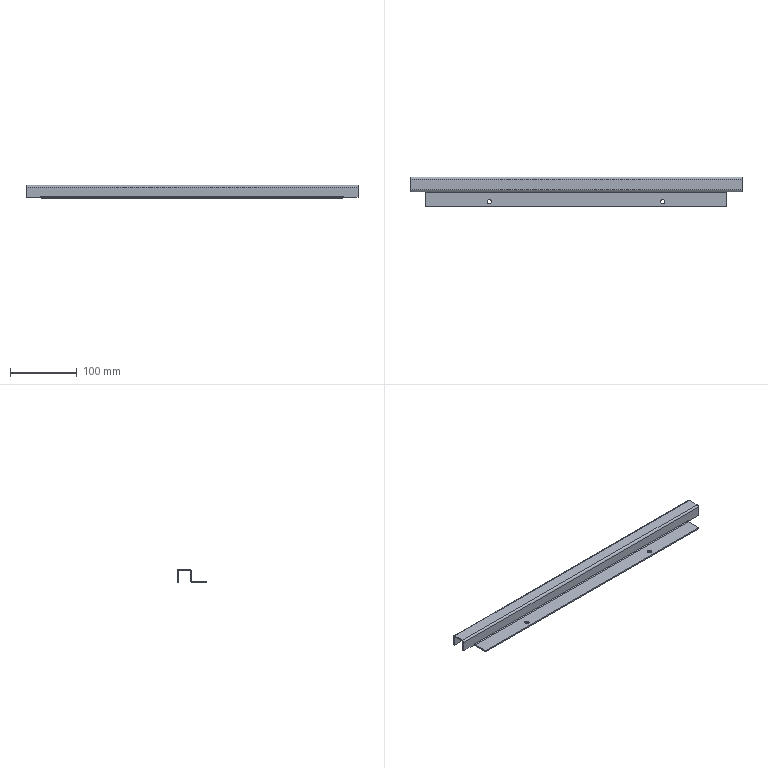Part | SolidWorks | features BaseBody 1 | 1 solid | 44 faces | box 498 x 44.9 x 20 mm | volume 75466 mm3 | plane 34 | cylinder 10 | commonest cylinder face diameters 6.5 x4 2 x3 6 x3
STEP:
#1=CARTESIAN_POINT('',(-226.,8.95,-18.));
#2=VERTEX_POINT('',#1);
#3=CARTESIAN_POINT('',(-226.,10.95,-18.));
#4=VERTEX_POINT('',#3);
#5=CARTESIAN_POINT('',(-226.,-33.95,-18.));
#6=DIRECTION('',(0.,1.,0.));
#7=VECTOR('',#6,1000.);
#8=LINE('',#5,#7);
#9=EDGE_CURVE('',#2,#4,#8,.T.);
#10=ORIENTED_EDGE('',*,*,#9,.T.);
#11=CARTESIAN_POINT('',(-226.,10.95,-20.));
#12=VERTEX_POINT('',#11);
#13=CARTESIAN_POINT('',(-226.,10.95,-20.));
#14=DIRECTION('',(0.,0.,-1.));
#15=VECTOR('',#14,1000.);
#16=LINE('',#13,#15);
#17=EDGE_CURVE('',#4,#12,#16,.T.);
#18=ORIENTED_EDGE('',*,*,#17,.T.);
#19=CARTESIAN_POINT('',(-226.,8.95,-20.));
#20=VERTEX_POINT('',#19);
#21=CARTESIAN_POINT('',(-226.,-33.95,-20.));
#22=DIRECTION('',(0.,1.,0.));
#23=VECTOR('',#22,1000.);
#24=LINE('',#21,#23);
#25=EDGE_CURVE('',#20,#12,#24,.T.);
#26=ORIENTED_EDGE('',*,*,#25,.F.);
#27=CARTESIAN_POINT('',(-226.,8.95,0.));
#28=DIRECTION('',(0.,0.,-1.));
#29=VECTOR('',#28,1000.);
#30=LINE('',#27,#29);
#31=EDGE_CURVE('',#2,#20,#30,.T.);
#32=ORIENTED_EDGE('',*,*,#31,.F.);
#33=EDGE_LOOP('',(#10,#18,#26,#32));
#34=FACE_OUTER_BOUND('',#33,.T.);
#35=CARTESIAN_POINT('',(-226.,-33.95,-20.));
#36=DIRECTION('',(1.,0.,0.));
#37=DIRECTION('',(0.,1.,0.));
#38=AXIS2_PLACEMENT_3D('',#35,#36,#37);
#39=PLANE('',#38);
#40=ADVANCED_FACE('',(#34),#39,.F.);
#41=CARTESIAN_POINT('',(-249.,8.95,-18.));
#42=VERTEX_POINT('',#41);
#43=CARTESIAN_POINT('',(-249.,10.95,-18.));
#44=VERTEX_POINT('',#43);
#45=CARTESIAN_POINT('',(-249.,-33.95,-18.));
#46=DIRECTION('',(0.,1.,0.));
#47=VECTOR('',#46,1000.);
#48=LINE('',#45,#47);
#49=EDGE_CURVE('',#42,#44,#48,.T.);
#50=ORIENTED_EDGE('',*,*,#49,.T.);
#51=CARTESIAN_POINT('',(-249.,10.95,-18.));
#52=DIRECTION('',(1.,0.,0.));
#53=VECTOR('',#52,1000.);
#54=LINE('',#51,#53);
#55=EDGE_CURVE('',#44,#4,#54,.T.);
#56=ORIENTED_EDGE('',*,*,#55,.T.);
#57=ORIENTED_EDGE('',*,*,#9,.F.);
#58=CARTESIAN_POINT('',(0.,8.95,-18.));
#59=DIRECTION('',(1.,0.,0.));
#60=VECTOR('',#59,1000.);
#61=LINE('',#58,#60);
#62=EDGE_CURVE('',#42,#2,#61,.T.);
#63=ORIENTED_EDGE('',*,*,#62,.F.);
#64=EDGE_LOOP('',(#50,#56,#57,#63));
#65=FACE_OUTER_BOUND('',#64,.T.);
#66=CARTESIAN_POINT('',(-249.,-33.95,-18.));
#67=DIRECTION('',(0.,0.,1.));
#68=DIRECTION('',(0.,-1.,0.));
#69=AXIS2_PLACEMENT_3D('',#66,#67,#68);
#70=PLANE('',#69);
#71=ADVANCED_FACE('',(#65),#70,.F.);
#72=CARTESIAN_POINT('',(226.,8.95,-20.));
#73=VERTEX_POINT('',#72);
#74=CARTESIAN_POINT('',(226.,10.95,-20.));
#75=VERTEX_POINT('',#74);
#76=CARTESIAN_POINT('',(226.,-33.95,-20.));
#77=DIRECTION('',(0.,1.,0.));
#78=VECTOR('',#77,1000.);
#79=LINE('',#76,#78);
#80=EDGE_CURVE('',#73,#75,#79,.T.);
#81=ORIENTED_EDGE('',*,*,#80,.T.);
#82=CARTESIAN_POINT('',(226.,10.95,-18.));
#83=VERTEX_POINT('',#82);
#84=CARTESIAN_POINT('',(226.,10.95,-20.));
#85=DIRECTION('',(0.,0.,1.));
#86=VECTOR('',#85,1000.);
#87=LINE('',#84,#86);
#88=EDGE_CURVE('',#75,#83,#87,.T.);
#89=ORIENTED_EDGE('',*,*,#88,.T.);
#90=CARTESIAN_POINT('',(226.,8.95,-18.));
#91=VERTEX_POINT('',#90);
#92=CARTESIAN_POINT('',(226.,-33.95,-18.));
#93=DIRECTION('',(0.,1.,0.));
#94=VECTOR('',#93,1000.);
#95=LINE('',#92,#94);
#96=EDGE_CURVE('',#91,#83,#95,.T.);
#97=ORIENTED_EDGE('',*,*,#96,.F.);
#98=CARTESIAN_POINT('',(226.,8.95,0.));
#99=DIRECTION('',(0.,0.,1.));
#100=VECTOR('',#99,1000.);
#101=LINE('',#98,#100);
#102=EDGE_CURVE('',#73,#91,#101,.T.);
#103=ORIENTED_EDGE('',*,*,#102,.F.);
#104=EDGE_LOOP('',(#81,#89,#97,#103));
#105=FACE_OUTER_BOUND('',#104,.T.);
#106=CARTESIAN_POINT('',(226.,-33.95,-20.));
#107=DIRECTION('',(-1.,0.,0.));
#108=DIRECTION('',(0.,0.,1.));
#109=AXIS2_PLACEMENT_3D('',#106,#107,#108);
#110=PLANE('',#109);
#111=ADVANCED_FACE('',(#105),#110,.F.);
#112=ORIENTED_EDGE('',*,*,#96,.T.);
#113=CARTESIAN_POINT('',(249.,10.95,-18.));
#114=VERTEX_POINT('',#113);
#115=CARTESIAN_POINT('',(249.,10.95,-18.));
#116=DIRECTION('',(1.,0.,0.));
#117=VECTOR('',#116,1000.);
#118=LINE('',#115,#117);
#119=EDGE_CURVE('',#83,#114,#118,.T.);
#120=ORIENTED_EDGE('',*,*,#119,.T.);
#121=CARTESIAN_POINT('',(249.,8.95,-18.));
#122=VERTEX_POINT('',#121);
#123=CARTESIAN_POINT('',(249.,-33.95,-18.));
#124=DIRECTION('',(0.,1.,0.));
#125=VECTOR('',#124,1000.);
#126=LINE('',#123,#125);
#127=EDGE_CURVE('',#122,#114,#126,.T.);
#128=ORIENTED_EDGE('',*,*,#127,.F.);
#129=CARTESIAN_POINT('',(0.,8.95,-18.));
#130=DIRECTION('',(1.,0.,0.));
#131=VECTOR('',#130,1000.);
#132=LINE('',#129,#131);
#133=EDGE_CURVE('',#91,#122,#132,.T.);
#134=ORIENTED_EDGE('',*,*,#133,.F.);
#135=EDGE_LOOP('',(#112,#120,#128,#134));
#136=FACE_OUTER_BOUND('',#135,.T.);
#137=CARTESIAN_POINT('',(249.,-33.95,-18.));
#138=DIRECTION('',(0.,0.,1.));
#139=DIRECTION('',(0.,-1.,0.));
#140=AXIS2_PLACEMENT_3D('',#137,#138,#139);
#141=PLANE('',#140);
#142=ADVANCED_FACE('',(#136),#141,.F.);
#143=CARTESIAN_POINT('',(227.,-10.95,-18.));
#144=VERTEX_POINT('',#143);
#145=CARTESIAN_POINT('',(227.,-8.95,-18.));
#146=VERTEX_POINT('',#145);
#147=CARTESIAN_POINT('',(227.,-10.95,-18.));
#148=DIRECTION('',(0.,1.,0.));
#149=VECTOR('',#148,1000.);
#150=LINE('',#147,#149);
#151=EDGE_CURVE('',#144,#146,#150,.T.);
#152=ORIENTED_EDGE('',*,*,#151,.T.);
#153=CARTESIAN_POINT('',(249.,-8.95,-18.));
#154=VERTEX_POINT('',#153);
#155=CARTESIAN_POINT('',(0.,-8.95,-18.));
#156=DIRECTION('',(1.,0.,0.));
#157=VECTOR('',#156,1000.);
#158=LINE('',#155,#157);
#159=EDGE_CURVE('',#146,#154,#158,.T.);
#160=ORIENTED_EDGE('',*,*,#159,.T.);
#161=CARTESIAN_POINT('',(249.,-10.95,-18.));
#162=VERTEX_POINT('',#161);
#163=CARTESIAN_POINT('',(249.,-33.95,-18.));
#164=DIRECTION('',(0.,1.,0.));
#165=VECTOR('',#164,1000.);
#166=LINE('',#163,#165);
#167=EDGE_CURVE('',#162,#154,#166,.T.);
#168=ORIENTED_EDGE('',*,*,#167,.F.);
#169=CARTESIAN_POINT('',(0.,-10.95,-18.));
#170=DIRECTION('',(1.,0.,0.));
#171=VECTOR('',#170,1000.);
#172=LINE('',#169,#171);
#173=EDGE_CURVE('',#144,#162,#172,.T.);
#174=ORIENTED_EDGE('',*,*,#173,.F.);
#175=EDGE_LOOP('',(#152,#160,#168,#174));
#176=FACE_OUTER_BOUND('',#175,.T.);
#177=CARTESIAN_POINT('',(249.,-33.95,-18.));
#178=DIRECTION('',(0.,0.,1.));
#179=DIRECTION('',(0.,-1.,0.));
#180=AXIS2_PLACEMENT_3D('',#177,#178,#179);
#181=PLANE('',#180);
#182=ADVANCED_FACE('',(#176),#181,.F.);
#183=CARTESIAN_POINT('',(-249.,-10.95,-18.));
#184=VERTEX_POINT('',#183);
#185=CARTESIAN_POINT('',(-249.,-8.95,-18.));
#186=VERTEX_POINT('',#185);
#187=CARTESIAN_POINT('',(-249.,-33.95,-18.));
#188=DIRECTION('',(0.,1.,0.));
#189=VECTOR('',#188,1000.);
#190=LINE('',#187,#189);
#191=EDGE_CURVE('',#184,#186,#190,.T.);
#192=ORIENTED_EDGE('',*,*,#191,.T.);
#193=CARTESIAN_POINT('',(-227.,-8.95,-18.));
#194=VERTEX_POINT('',#193);
#195=CARTESIAN_POINT('',(0.,-8.95,-18.));
#196=DIRECTION('',(1.,0.,0.));
#197=VECTOR('',#196,1000.);
#198=LINE('',#195,#197);
#199=EDGE_CURVE('',#186,#194,#198,.T.);
#200=ORIENTED_EDGE('',*,*,#199,.T.);
#201=CARTESIAN_POINT('',(-227.,-10.95,-18.));
#202=VERTEX_POINT('',#201);
#203=CARTESIAN_POINT('',(-227.,-10.95,-18.));
#204=DIRECTION('',(0.,-1.,0.));
#205=VECTOR('',#204,1000.);
#206=LINE('',#203,#205);
#207=EDGE_CURVE('',#194,#202,#206,.T.);
#208=ORIENTED_EDGE('',*,*,#207,.T.);
#209=CARTESIAN_POINT('',(0.,-10.95,-18.));
#210=DIRECTION('',(1.,0.,0.));
#211=VECTOR('',#210,1000.);
#212=LINE('',#209,#211);
#213=EDGE_CURVE('',#184,#202,#212,.T.);
#214=ORIENTED_EDGE('',*,*,#213,.F.);
#215=EDGE_LOOP('',(#192,#200,#208,#214));
#216=FACE_OUTER_BOUND('',#215,.T.);
#217=CARTESIAN_POINT('',(-249.,-33.95,-18.));
#218=DIRECTION('',(0.,0.,1.));
#219=DIRECTION('',(0.,-1.,0.));
#220=AXIS2_PLACEMENT_3D('',#217,#218,#219);
#221=PLANE('',#220);
#222=ADVANCED_FACE('',(#216),#221,.F.);
#223=CARTESIAN_POINT('',(-133.25,-25.95,-20.));
#224=VERTEX_POINT('',#223);
#225=CARTESIAN_POINT('',(-133.25,-25.95,-18.));
#226=VERTEX_POINT('',#225);
#227=CARTESIAN_POINT('',(-133.25,-25.95,-20.));
#228=DIRECTION('',(0.,0.,1.));
#229=VECTOR('',#228,1000.);
#230=LINE('',#227,#229);
#231=EDGE_CURVE('',#224,#226,#230,.T.);
#232=ORIENTED_EDGE('',*,*,#231,.F.);
#233=CARTESIAN_POINT('',(-126.75,-25.95,-20.));
#234=VERTEX_POINT('',#233);
#235=CARTESIAN_POINT('',(-130.,-25.95,-20.));
#236=DIRECTION('',(0.,0.,1.));
#237=DIRECTION('',(1.,0.,0.));
#238=AXIS2_PLACEMENT_3D('',#235,#236,#237);
#239=CIRCLE('',#238,3.25);
#240=EDGE_CURVE('',#234,#224,#239,.T.);
#241=ORIENTED_EDGE('',*,*,#240,.F.);
#242=CARTESIAN_POINT('',(-126.75,-25.95,-18.));
#243=VERTEX_POINT('',#242);
#244=CARTESIAN_POINT('',(-126.75,-25.95,-20.));
#245=DIRECTION('',(0.,0.,1.));
#246=VECTOR('',#245,1000.);
#247=LINE('',#244,#246);
#248=EDGE_CURVE('',#234,#243,#247,.T.);
#249=ORIENTED_EDGE('',*,*,#248,.T.);
#250=CARTESIAN_POINT('',(-130.,-25.95,-18.));
#251=DIRECTION('',(0.,0.,1.));
#252=DIRECTION('',(1.,0.,0.));
#253=AXIS2_PLACEMENT_3D('',#250,#251,#252);
#254=CIRCLE('',#253,3.25);
#255=EDGE_CURVE('',#243,#226,#254,.T.);
#256=ORIENTED_EDGE('',*,*,#255,.T.);
#257=EDGE_LOOP('',(#232,#241,#249,#256));
#258=FACE_OUTER_BOUND('',#257,.T.);
#259=CARTESIAN_POINT('',(-130.,-25.95,-20.));
#260=DIRECTION('',(0.,0.,1.));
#261=DIRECTION('',(1.,0.,0.));
#262=AXIS2_PLACEMENT_3D('',#259,#260,#261);
#263=CYLINDRICAL_SURFACE('',#262,3.25);
#264=ADVANCED_FACE('',(#258),#263,.F.);
#265=CARTESIAN_POINT('',(126.75,-25.95,-20.));
#266=VERTEX_POINT('',#265);
#267=CARTESIAN_POINT('',(126.75,-25.95,-18.));
#268=VERTEX_POINT('',#267);
#269=CARTESIAN_POINT('',(126.75,-25.95,-20.));
#270=DIRECTION('',(0.,0.,1.));
#271=VECTOR('',#270,1000.);
#272=LINE('',#269,#271);
#273=EDGE_CURVE('',#266,#268,#272,.T.);
#274=ORIENTED_EDGE('',*,*,#273,.F.);
#275=CARTESIAN_POINT('',(133.25,-25.95,-20.));
#276=VERTEX_POINT('',#275);
#277=CARTESIAN_POINT('',(130.,-25.95,-20.));
#278=DIRECTION('',(0.,0.,1.));
#279=DIRECTION('',(-1.,0.,0.));
#280=AXIS2_PLACEMENT_3D('',#277,#278,#279);
#281=CIRCLE('',#280,3.25);
#282=EDGE_CURVE('',#276,#266,#281,.T.);
#283=ORIENTED_EDGE('',*,*,#282,.F.);
#284=CARTESIAN_POINT('',(133.25,-25.95,-18.));
#285=VERTEX_POINT('',#284);
#286=CARTESIAN_POINT('',(133.25,-25.95,-20.));
#287=DIRECTION('',(0.,0.,1.));
#288=VECTOR('',#287,1000.);
#289=LINE('',#286,#288);
#290=EDGE_CURVE('',#276,#285,#289,.T.);
#291=ORIENTED_EDGE('',*,*,#290,.T.);
#292=CARTESIAN_POINT('',(130.,-25.95,-18.));
#293=DIRECTION('',(0.,0.,1.));
#294=DIRECTION('',(-1.,0.,0.));
#295=AXIS2_PLACEMENT_3D('',#292,#293,#294);
#296=CIRCLE('',#295,3.25);
#297=EDGE_CURVE('',#285,#268,#296,.T.);
#298=ORIENTED_EDGE('',*,*,#297,.T.);
#299=EDGE_LOOP('',(#274,#283,#291,#298));
#300=FACE_OUTER_BOUND('',#299,.T.);
#301=CARTESIAN_POINT('',(130.,-25.95,-20.));
#302=DIRECTION('',(0.,0.,1.));
#303=DIRECTION('',(1.,0.,0.));
#304=AXIS2_PLACEMENT_3D('',#301,#302,#303);
#305=CYLINDRICAL_SURFACE('',#304,3.25);
#306=ADVANCED_FACE('',(#300),#305,.F.);
#307=CARTESIAN_POINT('',(-226.,-33.95,-18.));
#308=VERTEX_POINT('',#307);
#309=CARTESIAN_POINT('',(226.,-33.95,-18.));
#310=VERTEX_POINT('',#309);
#311=CARTESIAN_POINT('',(0.,-33.95,-18.));
#312=DIRECTION('',(1.,0.,0.));
#313=VECTOR('',#312,1000.);
#314=LINE('',#311,#313);
#315=EDGE_CURVE('',#308,#310,#314,.T.);
#316=ORIENTED_EDGE('',*,*,#315,.F.);
#317=CARTESIAN_POINT('',(-226.,-33.95,-20.));
#318=VERTEX_POINT('',#317);
#319=CARTESIAN_POINT('',(-226.,-33.95,-20.));
#320=DIRECTION('',(0.,0.,1.));
#321=VECTOR('',#320,1000.);
#322=LINE('',#319,#321);
#323=EDGE_CURVE('',#318,#308,#322,.T.);
#324=ORIENTED_EDGE('',*,*,#323,.F.);
#325=CARTESIAN_POINT('',(226.,-33.95,-20.));
#326=VERTEX_POINT('',#325);
#327=CARTESIAN_POINT('',(-226.,-33.95,-20.));
#328=DIRECTION('',(1.,0.,0.));
#329=VECTOR('',#328,1000.);
#330=LINE('',#327,#329);
#331=EDGE_CURVE('',#318,#326,#330,.T.);
#332=ORIENTED_EDGE('',*,*,#331,.T.);
#333=CARTESIAN_POINT('',(226.,-33.95,-20.));
#334=DIRECTION('',(0.,0.,1.));
#335=VECTOR('',#334,1000.);
#336=LINE('',#333,#335);
#337=EDGE_CURVE('',#326,#310,#336,.T.);
#338=ORIENTED_EDGE('',*,*,#337,.T.);
#339=EDGE_LOOP('',(#316,#324,#332,#338));
#340=FACE_OUTER_BOUND('',#339,.T.);
#341=CARTESIAN_POINT('',(-226.,-33.95,-20.));
#342=DIRECTION('',(0.,-1.,0.));
#343=DIRECTION('',(0.,0.,-1.));
#344=AXIS2_PLACEMENT_3D('',#341,#342,#343);
#345=PLANE('',#344);
#346=ADVANCED_FACE('',(#340),#345,.T.);
#347=ORIENTED_EDGE('',*,*,#297,.F.);
#348=CARTESIAN_POINT('',(130.,-25.95,-18.));
#349=DIRECTION('',(0.,0.,1.));
#350=DIRECTION('',(-1.,0.,0.));
#351=AXIS2_PLACEMENT_3D('',#348,#349,#350);
#352=CIRCLE('',#351,3.25);
#353=EDGE_CURVE('',#268,#285,#352,.T.);
#354=ORIENTED_EDGE('',*,*,#353,.F.);
#355=EDGE_LOOP('',(#347,#354));
#356=FACE_BOUND('',#355,.T.);
#357=ORIENTED_EDGE('',*,*,#255,.F.);
#358=CARTESIAN_POINT('',(-130.,-25.95,-18.));
#359=DIRECTION('',(0.,0.,1.));
#360=DIRECTION('',(1.,0.,0.));
#361=AXIS2_PLACEMENT_3D('',#358,#359,#360);
#362=CIRCLE('',#361,3.25);
#363=EDGE_CURVE('',#226,#243,#362,.T.);
#364=ORIENTED_EDGE('',*,*,#363,.F.);
#365=EDGE_LOOP('',(#357,#364));
#366=FACE_BOUND('',#365,.T.);
#367=CARTESIAN_POINT('',(226.,-11.95,-18.));
#368=VERTEX_POINT('',#367);
#369=CARTESIAN_POINT('',(226.,0.,-18.));
#370=DIRECTION('',(0.,1.,0.));
#371=VECTOR('',#370,1000.);
#372=LINE('',#369,#371);
#373=EDGE_CURVE('',#310,#368,#372,.T.);
#374=ORIENTED_EDGE('',*,*,#373,.T.);
#375=CARTESIAN_POINT('',(-226.,-11.95,-18.));
#376=VERTEX_POINT('',#375);
#377=CARTESIAN_POINT('',(-226.,-11.95,-18.));
#378=DIRECTION('',(1.,0.,0.));
#379=VECTOR('',#378,1000.);
#380=LINE('',#377,#379);
#381=EDGE_CURVE('',#376,#368,#380,.T.);
#382=ORIENTED_EDGE('',*,*,#381,.F.);
#383=CARTESIAN_POINT('',(-226.,0.,-18.));
#384=DIRECTION('',(0.,-1.,0.));
#385=VECTOR('',#384,1000.);
#386=LINE('',#383,#385);
#387=EDGE_CURVE('',#376,#308,#386,.T.);
#388=ORIENTED_EDGE('',*,*,#387,.T.);
#389=ORIENTED_EDGE('',*,*,#315,.T.);
#390=EDGE_LOOP('',(#374,#382,#388,#389));
#391=FACE_OUTER_BOUND('',#390,.T.);
#392=CARTESIAN_POINT('',(0.,0.,-18.));
#393=DIRECTION('',(0.,0.,1.));
#394=DIRECTION('',(1.,0.,0.));
#395=AXIS2_PLACEMENT_3D('',#392,#393,#394);
#396=PLANE('',#395);
#397=ADVANCED_FACE('',(#356,#366,#391),#396,.T.);
#398=ORIENTED_EDGE('',*,*,#282,.T.);
#399=CARTESIAN_POINT('',(130.,-25.95,-20.));
#400=DIRECTION('',(0.,0.,1.));
#401=DIRECTION('',(-1.,0.,0.));
#402=AXIS2_PLACEMENT_3D('',#399,#400,#401);
#403=CIRCLE('',#402,3.25);
#404=EDGE_CURVE('',#266,#276,#403,.T.);
#405=ORIENTED_EDGE('',*,*,#404,.T.);
#406=EDGE_LOOP('',(#398,#405));
#407=FACE_BOUND('',#406,.T.);
#408=ORIENTED_EDGE('',*,*,#240,.T.);
#409=CARTESIAN_POINT('',(-130.,-25.95,-20.));
#410=DIRECTION('',(0.,0.,1.));
#411=DIRECTION('',(1.,0.,0.));
#412=AXIS2_PLACEMENT_3D('',#409,#410,#411);
#413=CIRCLE('',#412,3.25);
#414=EDGE_CURVE('',#224,#234,#413,.T.);
#415=ORIENTED_EDGE('',*,*,#414,.T.);
#416=EDGE_LOOP('',(#408,#415));
#417=FACE_BOUND('',#416,.T.);
#418=CARTESIAN_POINT('',(226.,-11.95,-20.));
#419=VERTEX_POINT('',#418);
#420=CARTESIAN_POINT('',(-226.,-11.95,-20.));
#421=VERTEX_POINT('',#420);
#422=CARTESIAN_POINT('',(-226.,-11.95,-20.));
#423=DIRECTION('',(-1.,0.,0.));
#424=VECTOR('',#423,1000.);
#425=LINE('',#422,#424);
#426=EDGE_CURVE('',#419,#421,#425,.T.);
#427=ORIENTED_EDGE('',*,*,#426,.F.);
#428=CARTESIAN_POINT('',(226.,-10.95,-20.));
#429=DIRECTION('',(0.,1.,0.));
#430=VECTOR('',#429,1000.);
#431=LINE('',#428,#430);
#432=EDGE_CURVE('',#326,#419,#431,.T.);
#433=ORIENTED_EDGE('',*,*,#432,.F.);
#434=ORIENTED_EDGE('',*,*,#331,.F.);
#435=CARTESIAN_POINT('',(-226.,-10.95,-20.));
#436=DIRECTION('',(0.,-1.,0.));
#437=VECTOR('',#436,1000.);
#438=LINE('',#435,#437);
#439=EDGE_CURVE('',#421,#318,#438,.T.);
#440=ORIENTED_EDGE('',*,*,#439,.F.);
#441=EDGE_LOOP('',(#427,#433,#434,#440));
#442=FACE_OUTER_BOUND('',#441,.T.);
#443=CARTESIAN_POINT('',(0.,0.,-20.));
#444=DIRECTION('',(0.,0.,1.));
#445=DIRECTION('',(1.,0.,0.));
#446=AXIS2_PLACEMENT_3D('',#443,#444,#445);
#447=PLANE('',#446);
#448=ADVANCED_FACE('',(#407,#417,#442),#447,.F.);
#449=CARTESIAN_POINT('',(226.,-10.95,-17.));
#450=VERTEX_POINT('',#449);
#451=CARTESIAN_POINT('',(-226.,-10.95,-17.));
#452=VERTEX_POINT('',#451);
#453=CARTESIAN_POINT('',(226.,-10.95,-17.));
#454=DIRECTION('',(-1.,0.,0.));
#455=VECTOR('',#454,1000.);
#456=LINE('',#453,#455);
#457=EDGE_CURVE('',#450,#452,#456,.T.);
#458=ORIENTED_EDGE('',*,*,#457,.T.);
#459=CARTESIAN_POINT('',(-226.,-11.95,-17.));
#460=DIRECTION('',(-1.,0.,0.));
#461=DIRECTION('',(0.,0.,-1.));
#462=AXIS2_PLACEMENT_3D('',#459,#460,#461);
#463=CIRCLE('',#462,1.);
#464=EDGE_CURVE('',#452,#376,#463,.T.);
#465=ORIENTED_EDGE('',*,*,#464,.T.);
#466=ORIENTED_EDGE('',*,*,#381,.T.);
#467=CARTESIAN_POINT('',(226.,-11.95,-17.));
#468=DIRECTION('',(1.,0.,0.));
#469=DIRECTION('',(0.,0.,-1.));
#470=AXIS2_PLACEMENT_3D('',#467,#468,#469);
#471=CIRCLE('',#470,1.);
#472=EDGE_CURVE('',#368,#450,#471,.T.);
#473=ORIENTED_EDGE('',*,*,#472,.T.);
#474=EDGE_LOOP('',(#458,#465,#466,#473));
#475=FACE_OUTER_BOUND('',#474,.T.);
#476=CARTESIAN_POINT('',(226.,-11.95,-17.));
#477=DIRECTION('',(1.,0.,0.));
#478=DIRECTION('',(0.,0.,-1.));
#479=AXIS2_PLACEMENT_3D('',#476,#477,#478);
#480=CYLINDRICAL_SURFACE('',#479,1.);
#481=ADVANCED_FACE('',(#475),#480,.F.);
#482=CARTESIAN_POINT('',(226.,-8.95,-17.));
#483=VERTEX_POINT('',#482);
#484=CARTESIAN_POINT('',(-226.,-8.95,-17.));
#485=VERTEX_POINT('',#484);
#486=CARTESIAN_POINT('',(226.,-8.95,-17.));
#487=DIRECTION('',(-1.,0.,0.));
#488=VECTOR('',#487,1000.);
#489=LINE('',#486,#488);
#490=EDGE_CURVE('',#483,#485,#489,.T.);
#491=ORIENTED_EDGE('',*,*,#490,.F.);
#492=CARTESIAN_POINT('',(226.,-11.95,-17.));
#493=DIRECTION('',(1.,0.,0.));
#494=DIRECTION('',(0.,0.,-1.));
#495=AXIS2_PLACEMENT_3D('',#492,#493,#494);
#496=CIRCLE('',#495,3.);
#497=EDGE_CURVE('',#419,#483,#496,.T.);
#498=ORIENTED_EDGE('',*,*,#497,.F.);
#499=ORIENTED_EDGE('',*,*,#426,.T.);
#500=CARTESIAN_POINT('',(-226.,-11.95,-17.));
#501=DIRECTION('',(-1.,0.,0.));
#502=DIRECTION('',(0.,0.,-1.));
#503=AXIS2_PLACEMENT_3D('',#500,#501,#502);
#504=CIRCLE('',#503,3.);
#505=EDGE_CURVE('',#485,#421,#504,.T.);
#506=ORIENTED_EDGE('',*,*,#505,.F.);
#507=EDGE_LOOP('',(#491,#498,#499,#506));
#508=FACE_OUTER_BOUND('',#507,.T.);
#509=CARTESIAN_POINT('',(226.,-11.95,-17.));
#510=DIRECTION('',(1.,0.,0.));
#511=DIRECTION('',(0.,0.,-1.));
#512=AXIS2_PLACEMENT_3D('',#509,#510,#511);
#513=CYLINDRICAL_SURFACE('',#512,3.);
#514=ADVANCED_FACE('',(#508),#513,.T.);
#515=ORIENTED_EDGE('',*,*,#472,.F.);
#516=ORIENTED_EDGE('',*,*,#373,.F.);
#517=ORIENTED_EDGE('',*,*,#337,.F.);
#518=ORIENTED_EDGE('',*,*,#432,.T.);
#519=ORIENTED_EDGE('',*,*,#497,.T.);
#520=CARTESIAN_POINT('',(226.,-10.95,-17.));
#521=DIRECTION('',(0.,1.,0.));
#522=VECTOR('',#521,1000.);
#523=LINE('',#520,#522);
#524=EDGE_CURVE('',#450,#483,#523,.T.);
#525=ORIENTED_EDGE('',*,*,#524,.F.);
#526=EDGE_LOOP('',(#515,#516,#517,#518,#519,#525));
#527=FACE_OUTER_BOUND('',#526,.T.);
#528=CARTESIAN_POINT('',(226.,-11.95,-17.));
#529=DIRECTION('',(-1.,0.,0.));
#530=DIRECTION('',(0.,0.,1.));
#531=AXIS2_PLACEMENT_3D('',#528,#529,#530);
#532=PLANE('',#531);
#533=ADVANCED_FACE('',(#527),#532,.F.);
#534=ORIENTED_EDGE('',*,*,#505,.T.);
#535=ORIENTED_EDGE('',*,*,#439,.T.);
#536=ORIENTED_EDGE('',*,*,#323,.T.);
#537=ORIENTED_EDGE('',*,*,#387,.F.);
#538=ORIENTED_EDGE('',*,*,#464,.F.);
#539=CARTESIAN_POINT('',(-226.,-10.95,-17.));
#540=DIRECTION('',(0.,1.,0.));
#541=VECTOR('',#540,1000.);
#542=LINE('',#539,#541);
#543=EDGE_CURVE('',#452,#485,#542,.T.);
#544=ORIENTED_EDGE('',*,*,#543,.T.);
#545=EDGE_LOOP('',(#534,#535,#536,#537,#538,#544));
#546=FACE_OUTER_BOUND('',#545,.T.);
#547=CARTESIAN_POINT('',(-226.,-11.95,-17.));
#548=DIRECTION('',(-1.,0.,0.));
#549=DIRECTION('',(0.,0.,1.));
#550=AXIS2_PLACEMENT_3D('',#547,#548,#549);
#551=PLANE('',#550);
#552=ADVANCED_FACE('',(#546),#551,.T.);
#553=ORIENTED_EDGE('',*,*,#207,.F.);
#554=CARTESIAN_POINT('',(-227.,-8.95,-16.));
#555=VERTEX_POINT('',#554);
#556=CARTESIAN_POINT('',(-227.,-8.95,0.));
#557=DIRECTION('',(0.,0.,-1.));
#558=VECTOR('',#557,1000.);
#559=LINE('',#556,#558);
#560=EDGE_CURVE('',#555,#194,#559,.T.);
#561=ORIENTED_EDGE('',*,*,#560,.F.);
#562=CARTESIAN_POINT('',(-227.,-10.95,-16.));
#563=VERTEX_POINT('',#562);
#564=CARTESIAN_POINT('',(-227.,-10.95,-16.));
#565=DIRECTION('',(0.,1.,0.));
#566=VECTOR('',#565,1000.);
#567=LINE('',#564,#566);
#568=EDGE_CURVE('',#563,#555,#567,.T.);
#569=ORIENTED_EDGE('',*,*,#568,.F.);
#570=CARTESIAN_POINT('',(-227.,-10.95,-16.));
#571=DIRECTION('',(0.,0.,-1.));
#572=VECTOR('',#571,1000.);
#573=LINE('',#570,#572);
#574=EDGE_CURVE('',#563,#202,#573,.T.);
#575=ORIENTED_EDGE('',*,*,#574,.T.);
#576=EDGE_LOOP('',(#553,#561,#569,#575));
#577=FACE_OUTER_BOUND('',#576,.T.);
#578=CARTESIAN_POINT('',(-227.,-10.95,-16.));
#579=DIRECTION('',(1.,0.,0.));
#580=DIRECTION('',(0.,0.,1.));
#581=AXIS2_PLACEMENT_3D('',#578,#579,#580);
#582=PLANE('',#581);
#583=ADVANCED_FACE('',(#577),#582,.T.);
#584=CARTESIAN_POINT('',(-226.,-8.95,-16.));
#585=VERTEX_POINT('',#584);
#586=CARTESIAN_POINT('',(0.,-8.95,-16.));
#587=DIRECTION('',(-1.,0.,0.));
#588=VECTOR('',#587,1000.);
#589=LINE('',#586,#588);
#590=EDGE_CURVE('',#585,#555,#589,.T.);
#591=ORIENTED_EDGE('',*,*,#590,.F.);
#592=CARTESIAN_POINT('',(-226.,-10.95,-16.));
#593=VERTEX_POINT('',#592);
#594=CARTESIAN_POINT('',(-226.,-10.95,-16.));
#595=DIRECTION('',(0.,1.,0.));
#596=VECTOR('',#595,1000.);
#597=LINE('',#594,#596);
#598=EDGE_CURVE('',#593,#585,#597,.T.);
#599=ORIENTED_EDGE('',*,*,#598,.F.);
#600=CARTESIAN_POINT('',(-226.,-10.95,-16.));
#601=DIRECTION('',(-1.,0.,0.));
#602=VECTOR('',#601,1000.);
#603=LINE('',#600,#602);
#604=EDGE_CURVE('',#593,#563,#603,.T.);
#605=ORIENTED_EDGE('',*,*,#604,.T.);
#606=ORIENTED_EDGE('',*,*,#568,.T.);
#607=EDGE_LOOP('',(#591,#599,#605,#606));
#608=FACE_OUTER_BOUND('',#607,.T.);
#609=CARTESIAN_POINT('',(-226.,-10.95,-16.));
#610=DIRECTION('',(0.,0.,-1.));
#611=DIRECTION('',(0.,-1.,0.));
#612=AXIS2_PLACEMENT_3D('',#609,#610,#611);
#613=PLANE('',#612);
#614=ADVANCED_FACE('',(#608),#613,.T.);
#615=CARTESIAN_POINT('',(-226.,-8.95,0.));
#616=DIRECTION('',(0.,0.,1.));
#617=VECTOR('',#616,1000.);
#618=LINE('',#615,#617);
#619=EDGE_CURVE('',#485,#585,#618,.T.);
#620=ORIENTED_EDGE('',*,*,#619,.F.);
#621=ORIENTED_EDGE('',*,*,#543,.F.);
#622=CARTESIAN_POINT('',(-226.,-10.95,-17.));
#623=DIRECTION('',(0.,0.,1.));
#624=VECTOR('',#623,1000.);
#625=LINE('',#622,#624);
#626=EDGE_CURVE('',#452,#593,#625,.T.);
#627=ORIENTED_EDGE('',*,*,#626,.T.);
#628=ORIENTED_EDGE('',*,*,#598,.T.);
#629=EDGE_LOOP('',(#620,#621,#627,#628));
#630=FACE_OUTER_BOUND('',#629,.T.);
#631=CARTESIAN_POINT('',(-226.,-10.95,-17.));
#632=DIRECTION('',(-1.,0.,0.));
#633=DIRECTION('',(0.,1.,0.));
#634=AXIS2_PLACEMENT_3D('',#631,#632,#633);
#635=PLANE('',#634);
#636=ADVANCED_FACE('',(#630),#635,.T.);
#637=CARTESIAN_POINT('',(226.,-8.95,-16.));
#638=VERTEX_POINT('',#637);
#639=CARTESIAN_POINT('',(226.,-8.95,0.));
#640=DIRECTION('',(0.,0.,-1.));
#641=VECTOR('',#640,1000.);
#642=LINE('',#639,#641);
#643=EDGE_CURVE('',#638,#483,#642,.T.);
#644=ORIENTED_EDGE('',*,*,#643,.F.);
#645=CARTESIAN_POINT('',(226.,-10.95,-16.));
#646=VERTEX_POINT('',#645);
#647=CARTESIAN_POINT('',(226.,-10.95,-16.));
#648=DIRECTION('',(0.,1.,0.));
#649=VECTOR('',#648,1000.);
#650=LINE('',#647,#649);
#651=EDGE_CURVE('',#646,#638,#650,.T.);
#652=ORIENTED_EDGE('',*,*,#651,.F.);
#653=CARTESIAN_POINT('',(226.,-10.95,-16.));
#654=DIRECTION('',(0.,0.,-1.));
#655=VECTOR('',#654,1000.);
#656=LINE('',#653,#655);
#657=EDGE_CURVE('',#646,#450,#656,.T.);
#658=ORIENTED_EDGE('',*,*,#657,.T.);
#659=ORIENTED_EDGE('',*,*,#524,.T.);
#660=EDGE_LOOP('',(#644,#652,#658,#659));
#661=FACE_OUTER_BOUND('',#660,.T.);
#662=CARTESIAN_POINT('',(226.,-10.95,-16.));
#663=DIRECTION('',(1.,0.,0.));
#664=DIRECTION('',(0.,1.,0.));
#665=AXIS2_PLACEMENT_3D('',#662,#663,#664);
#666=PLANE('',#665);
#667=ADVANCED_FACE('',(#661),#666,.T.);
#668=CARTESIAN_POINT('',(227.,-8.95,-16.));
#669=VERTEX_POINT('',#668);
#670=CARTESIAN_POINT('',(0.,-8.95,-16.));
#671=DIRECTION('',(-1.,0.,0.));
#672=VECTOR('',#671,1000.);
#673=LINE('',#670,#672);
#674=EDGE_CURVE('',#669,#638,#673,.T.);
#675=ORIENTED_EDGE('',*,*,#674,.F.);
#676=CARTESIAN_POINT('',(227.,-10.95,-16.));
#677=VERTEX_POINT('',#676);
#678=CARTESIAN_POINT('',(227.,-10.95,-16.));
#679=DIRECTION('',(0.,1.,0.));
#680=VECTOR('',#679,1000.);
#681=LINE('',#678,#680);
#682=EDGE_CURVE('',#677,#669,#681,.T.);
#683=ORIENTED_EDGE('',*,*,#682,.F.);
#684=CARTESIAN_POINT('',(227.,-10.95,-16.));
#685=DIRECTION('',(-1.,0.,0.));
#686=VECTOR('',#685,1000.);
#687=LINE('',#684,#686);
#688=EDGE_CURVE('',#677,#646,#687,.T.);
#689=ORIENTED_EDGE('',*,*,#688,.T.);
#690=ORIENTED_EDGE('',*,*,#651,.T.);
#691=EDGE_LOOP('',(#675,#683,#689,#690));
#692=FACE_OUTER_BOUND('',#691,.T.);
#693=CARTESIAN_POINT('',(227.,-10.95,-16.));
#694=DIRECTION('',(0.,0.,-1.));
#695=DIRECTION('',(0.,-1.,0.));
#696=AXIS2_PLACEMENT_3D('',#693,#694,#695);
#697=PLANE('',#696);
#698=ADVANCED_FACE('',(#692),#697,.T.);
#699=ORIENTED_EDGE('',*,*,#151,.F.);
#700=CARTESIAN_POINT('',(227.,-10.95,-20.));
#701=DIRECTION('',(0.,0.,1.));
#702=VECTOR('',#701,1000.);
#703=LINE('',#700,#702);
#704=EDGE_CURVE('',#144,#677,#703,.T.);
#705=ORIENTED_EDGE('',*,*,#704,.T.);
#706=ORIENTED_EDGE('',*,*,#682,.T.);
#707=CARTESIAN_POINT('',(227.,-8.95,0.));
#708=DIRECTION('',(0.,0.,1.));
#709=VECTOR('',#708,1000.);
#710=LINE('',#707,#709);
#711=EDGE_CURVE('',#146,#669,#710,.T.);
#712=ORIENTED_EDGE('',*,*,#711,.F.);
#713=EDGE_LOOP('',(#699,#705,#706,#712));
#714=FACE_OUTER_BOUND('',#713,.T.);
#715=CARTESIAN_POINT('',(227.,-10.95,-20.));
#716=DIRECTION('',(-1.,0.,0.));
#717=DIRECTION('',(0.,1.,0.));
#718=AXIS2_PLACEMENT_3D('',#715,#716,#717);
#719=PLANE('',#718);
#720=ADVANCED_FACE('',(#714),#719,.T.);
#721=ORIENTED_EDGE('',*,*,#191,.F.);
#722=CARTESIAN_POINT('',(-249.,-10.95,-3.));
#723=VERTEX_POINT('',#722);
#724=CARTESIAN_POINT('',(-249.,-10.95,-20.));
#725=DIRECTION('',(0.,0.,1.));
#726=VECTOR('',#725,1000.);
#727=LINE('',#724,#726);
#728=EDGE_CURVE('',#184,#723,#727,.T.);
#729=ORIENTED_EDGE('',*,*,#728,.T.);
#730=CARTESIAN_POINT('',(-249.,-8.95,-3.));
#731=VERTEX_POINT('',#730);
#732=CARTESIAN_POINT('',(-249.,-8.95,-3.));
#733=DIRECTION('',(0.,-1.,0.));
#734=VECTOR('',#733,1000.);
#735=LINE('',#732,#734);
#736=EDGE_CURVE('',#731,#723,#735,.T.);
#737=ORIENTED_EDGE('',*,*,#736,.F.);
#738=CARTESIAN_POINT('',(-249.,-8.95,0.));
#739=DIRECTION('',(0.,0.,1.));
#740=VECTOR('',#739,1000.);
#741=LINE('',#738,#740);
#742=EDGE_CURVE('',#186,#731,#741,.T.);
#743=ORIENTED_EDGE('',*,*,#742,.F.);
#744=EDGE_LOOP('',(#721,#729,#737,#743));
#745=FACE_OUTER_BOUND('',#744,.T.);
#746=CARTESIAN_POINT('',(-249.,-10.95,-20.));
#747=DIRECTION('',(-1.,0.,0.));
#748=DIRECTION('',(0.,1.,0.));
#749=AXIS2_PLACEMENT_3D('',#746,#747,#748);
#750=PLANE('',#749);
#751=ADVANCED_FACE('',(#745),#750,.T.);
#752=ORIENTED_EDGE('',*,*,#167,.T.);
#753=CARTESIAN_POINT('',(249.,-8.95,-3.));
#754=VERTEX_POINT('',#753);
#755=CARTESIAN_POINT('',(249.,-8.95,0.));
#756=DIRECTION('',(0.,0.,-1.));
#757=VECTOR('',#756,1000.);
#758=LINE('',#755,#757);
#759=EDGE_CURVE('',#754,#154,#758,.T.);
#760=ORIENTED_EDGE('',*,*,#759,.F.);
#761=CARTESIAN_POINT('',(249.,-10.95,-3.));
#762=VERTEX_POINT('',#761);
#763=CARTESIAN_POINT('',(249.,-10.95,-3.));
#764=DIRECTION('',(0.,-1.,0.));
#765=VECTOR('',#764,1000.);
#766=LINE('',#763,#765);
#767=EDGE_CURVE('',#754,#762,#766,.T.);
#768=ORIENTED_EDGE('',*,*,#767,.T.);
#769=CARTESIAN_POINT('',(249.,-10.95,-2.));
#770=DIRECTION('',(0.,0.,-1.));
#771=VECTOR('',#770,1000.);
#772=LINE('',#769,#771);
#773=EDGE_CURVE('',#762,#162,#772,.T.);
#774=ORIENTED_EDGE('',*,*,#773,.T.);
#775=EDGE_LOOP('',(#752,#760,#768,#774));
#776=FACE_OUTER_BOUND('',#775,.T.);
#777=CARTESIAN_POINT('',(249.,-10.95,-2.));
#778=DIRECTION('',(1.,0.,0.));
#779=DIRECTION('',(0.,0.,-1.));
#780=AXIS2_PLACEMENT_3D('',#777,#778,#779);
#781=PLANE('',#780);
#782=ADVANCED_FACE('',(#776),#781,.T.);
#783=CARTESIAN_POINT('',(-249.,-7.95,-2.));
#784=VERTEX_POINT('',#783);
#785=CARTESIAN_POINT('',(249.,-7.95,-2.));
#786=VERTEX_POINT('',#785);
#787=CARTESIAN_POINT('',(-249.,-7.95,-2.));
#788=DIRECTION('',(1.,0.,0.));
#789=VECTOR('',#788,1000.);
#790=LINE('',#787,#789);
#791=EDGE_CURVE('',#784,#786,#790,.T.);
#792=ORIENTED_EDGE('',*,*,#791,.T.);
#793=CARTESIAN_POINT('',(249.,-7.95,-3.));
#794=DIRECTION('',(1.,0.,0.));
#795=DIRECTION('',(0.,0.,1.));
#796=AXIS2_PLACEMENT_3D('',#793,#794,#795);
#797=CIRCLE('',#796,1.);
#798=EDGE_CURVE('',#786,#754,#797,.T.);
#799=ORIENTED_EDGE('',*,*,#798,.T.);
#800=CARTESIAN_POINT('',(249.,-8.95,-3.));
#801=DIRECTION('',(-1.,0.,0.));
#802=VECTOR('',#801,1000.);
#803=LINE('',#800,#802);
#804=EDGE_CURVE('',#754,#731,#803,.T.);
#805=ORIENTED_EDGE('',*,*,#804,.T.);
#806=CARTESIAN_POINT('',(-249.,-7.95,-3.));
#807=DIRECTION('',(-1.,0.,0.));
#808=DIRECTION('',(0.,0.,1.));
#809=AXIS2_PLACEMENT_3D('',#806,#807,#808);
#810=CIRCLE('',#809,1.);
#811=EDGE_CURVE('',#731,#784,#810,.T.);
#812=ORIENTED_EDGE('',*,*,#811,.T.);
#813=EDGE_LOOP('',(#792,#799,#805,#812));
#814=FACE_OUTER_BOUND('',#813,.T.);
#815=CARTESIAN_POINT('',(-249.,-7.95,-3.));
#816=DIRECTION('',(-1.,0.,0.));
#817=DIRECTION('',(0.,-1.,0.));
#818=AXIS2_PLACEMENT_3D('',#815,#816,#817);
#819=CYLINDRICAL_SURFACE('',#818,1.);
#820=ADVANCED_FACE('',(#814),#819,.F.);
#821=CARTESIAN_POINT('',(-249.,-7.95,0.));
#822=VERTEX_POINT('',#821);
#823=CARTESIAN_POINT('',(249.,-7.95,0.));
#824=VERTEX_POINT('',#823);
#825=CARTESIAN_POINT('',(-249.,-7.95,0.));
#826=DIRECTION('',(1.,0.,0.));
#827=VECTOR('',#826,1000.);
#828=LINE('',#825,#827);
#829=EDGE_CURVE('',#822,#824,#828,.T.);
#830=ORIENTED_EDGE('',*,*,#829,.F.);
#831=CARTESIAN_POINT('',(-249.,-7.95,-3.));
#832=DIRECTION('',(-1.,0.,0.));
#833=DIRECTION('',(0.,0.,1.));
#834=AXIS2_PLACEMENT_3D('',#831,#832,#833);
#835=CIRCLE('',#834,3.);
#836=EDGE_CURVE('',#723,#822,#835,.T.);
#837=ORIENTED_EDGE('',*,*,#836,.F.);
#838=CARTESIAN_POINT('',(249.,-10.95,-3.));
#839=DIRECTION('',(1.,0.,0.));
#840=VECTOR('',#839,1000.);
#841=LINE('',#838,#840);
#842=EDGE_CURVE('',#723,#762,#841,.T.);
#843=ORIENTED_EDGE('',*,*,#842,.T.);
#844=CARTESIAN_POINT('',(249.,-7.95,-3.));
#845=DIRECTION('',(1.,0.,0.));
#846=DIRECTION('',(0.,0.,1.));
#847=AXIS2_PLACEMENT_3D('',#844,#845,#846);
#848=CIRCLE('',#847,3.);
#849=EDGE_CURVE('',#824,#762,#848,.T.);
#850=ORIENTED_EDGE('',*,*,#849,.F.);
#851=EDGE_LOOP('',(#830,#837,#843,#850));
#852=FACE_OUTER_BOUND('',#851,.T.);
#853=CARTESIAN_POINT('',(-249.,-7.95,-3.));
#854=DIRECTION('',(-1.,0.,0.));
#855=DIRECTION('',(0.,-1.,0.));
#856=AXIS2_PLACEMENT_3D('',#853,#854,#855);
#857=CYLINDRICAL_SURFACE('',#856,3.);
#858=ADVANCED_FACE('',(#852),#857,.T.);
#859=ORIENTED_EDGE('',*,*,#811,.F.);
#860=ORIENTED_EDGE('',*,*,#736,.T.);
#861=ORIENTED_EDGE('',*,*,#836,.T.);
#862=CARTESIAN_POINT('',(-249.,-7.95,-2.));
#863=DIRECTION('',(0.,0.,1.));
#864=VECTOR('',#863,1000.);
#865=LINE('',#862,#864);
#866=EDGE_CURVE('',#784,#822,#865,.T.);
#867=ORIENTED_EDGE('',*,*,#866,.F.);
#868=EDGE_LOOP('',(#859,#860,#861,#867));
#869=FACE_OUTER_BOUND('',#868,.T.);
#870=CARTESIAN_POINT('',(-249.,-7.95,-3.));
#871=DIRECTION('',(1.,0.,0.));
#872=DIRECTION('',(0.,1.,0.));
#873=AXIS2_PLACEMENT_3D('',#870,#871,#872);
#874=PLANE('',#873);
#875=ADVANCED_FACE('',(#869),#874,.F.);
#876=ORIENTED_EDGE('',*,*,#767,.F.);
#877=ORIENTED_EDGE('',*,*,#798,.F.);
#878=CARTESIAN_POINT('',(249.,-7.95,-2.));
#879=DIRECTION('',(0.,0.,1.));
#880=VECTOR('',#879,1000.);
#881=LINE('',#878,#880);
#882=EDGE_CURVE('',#786,#824,#881,.T.);
#883=ORIENTED_EDGE('',*,*,#882,.T.);
#884=ORIENTED_EDGE('',*,*,#849,.T.);
#885=EDGE_LOOP('',(#876,#877,#883,#884));
#886=FACE_OUTER_BOUND('',#885,.T.);
#887=CARTESIAN_POINT('',(249.,-7.95,-3.));
#888=DIRECTION('',(1.,0.,0.));
#889=DIRECTION('',(0.,1.,0.));
#890=AXIS2_PLACEMENT_3D('',#887,#888,#889);
#891=PLANE('',#890);
#892=ADVANCED_FACE('',(#886),#891,.T.);
#893=ORIENTED_EDGE('',*,*,#25,.T.);
#894=CARTESIAN_POINT('',(249.,10.95,-20.));
#895=DIRECTION('',(1.,0.,0.));
#896=VECTOR('',#895,1000.);
#897=LINE('',#894,#896);
#898=EDGE_CURVE('',#12,#75,#897,.T.);
#899=ORIENTED_EDGE('',*,*,#898,.T.);
#900=ORIENTED_EDGE('',*,*,#80,.F.);
#901=CARTESIAN_POINT('',(0.,8.95,-20.));
#902=DIRECTION('',(1.,0.,0.));
#903=VECTOR('',#902,1000.);
#904=LINE('',#901,#903);
#905=EDGE_CURVE('',#20,#73,#904,.T.);
#906=ORIENTED_EDGE('',*,*,#905,.F.);
#907=EDGE_LOOP('',(#893,#899,#900,#906));
#908=FACE_OUTER_BOUND('',#907,.T.);
#909=CARTESIAN_POINT('',(249.,10.95,-20.));
#910=DIRECTION('',(0.,0.,-1.));
#911=DIRECTION('',(-1.,0.,0.));
#912=AXIS2_PLACEMENT_3D('',#909,#910,#911);
#913=PLANE('',#912);
#914=ADVANCED_FACE('',(#908),#913,.T.);
#915=ORIENTED_EDGE('',*,*,#62,.T.);
#916=ORIENTED_EDGE('',*,*,#31,.T.);
#917=ORIENTED_EDGE('',*,*,#905,.T.);
#918=ORIENTED_EDGE('',*,*,#102,.T.);
#919=ORIENTED_EDGE('',*,*,#133,.T.);
#920=CARTESIAN_POINT('',(249.,8.95,-3.));
#921=VERTEX_POINT('',#920);
#922=CARTESIAN_POINT('',(249.,8.95,0.));
#923=DIRECTION('',(0.,0.,1.));
#924=VECTOR('',#923,1000.);
#925=LINE('',#922,#924);
#926=EDGE_CURVE('',#122,#921,#925,.T.);
#927=ORIENTED_EDGE('',*,*,#926,.T.);
#928=CARTESIAN_POINT('',(-249.,8.95,-3.));
#929=VERTEX_POINT('',#928);
#930=CARTESIAN_POINT('',(-249.,8.95,-3.));
#931=DIRECTION('',(1.,0.,0.));
#932=VECTOR('',#931,1000.);
#933=LINE('',#930,#932);
#934=EDGE_CURVE('',#929,#921,#933,.T.);
#935=ORIENTED_EDGE('',*,*,#934,.F.);
#936=CARTESIAN_POINT('',(-249.,8.95,0.));
#937=DIRECTION('',(0.,0.,-1.));
#938=VECTOR('',#937,1000.);
#939=LINE('',#936,#938);
#940=EDGE_CURVE('',#929,#42,#939,.T.);
#941=ORIENTED_EDGE('',*,*,#940,.T.);
#942=EDGE_LOOP('',(#915,#916,#917,#918,#919,#927,#935,#941));
#943=FACE_OUTER_BOUND('',#942,.T.);
#944=CARTESIAN_POINT('',(0.,8.95,0.));
#945=DIRECTION('',(0.,1.,0.));
#946=DIRECTION('',(0.,0.,-1.));
#947=AXIS2_PLACEMENT_3D('',#944,#945,#946);
#948=PLANE('',#947);
#949=ADVANCED_FACE('',(#943),#948,.F.);
#950=ORIENTED_EDGE('',*,*,#17,.F.);
#951=ORIENTED_EDGE('',*,*,#55,.F.);
#952=CARTESIAN_POINT('',(-249.,10.95,-3.));
#953=VERTEX_POINT('',#952);
#954=CARTESIAN_POINT('',(-249.,10.95,-20.));
#955=DIRECTION('',(0.,0.,-1.));
#956=VECTOR('',#955,1000.);
#957=LINE('',#954,#956);
#958=EDGE_CURVE('',#953,#44,#957,.T.);
#959=ORIENTED_EDGE('',*,*,#958,.F.);
#960=CARTESIAN_POINT('',(249.,10.95,-3.));
#961=VERTEX_POINT('',#960);
#962=CARTESIAN_POINT('',(0.,10.95,-3.));
#963=DIRECTION('',(1.,0.,0.));
#964=VECTOR('',#963,1000.);
#965=LINE('',#962,#964);
#966=EDGE_CURVE('',#953,#961,#965,.T.);
#967=ORIENTED_EDGE('',*,*,#966,.T.);
#968=CARTESIAN_POINT('',(249.,10.95,-2.));
#969=DIRECTION('',(0.,0.,1.));
#970=VECTOR('',#969,1000.);
#971=LINE('',#968,#970);
#972=EDGE_CURVE('',#114,#961,#971,.T.);
#973=ORIENTED_EDGE('',*,*,#972,.F.);
#974=ORIENTED_EDGE('',*,*,#119,.F.);
#975=ORIENTED_EDGE('',*,*,#88,.F.);
#976=ORIENTED_EDGE('',*,*,#898,.F.);
#977=EDGE_LOOP('',(#950,#951,#959,#967,#973,#974,#975,#976));
#978=FACE_OUTER_BOUND('',#977,.T.);
#979=CARTESIAN_POINT('',(0.,10.95,0.));
#980=DIRECTION('',(0.,1.,0.));
#981=DIRECTION('',(0.,0.,-1.));
#982=AXIS2_PLACEMENT_3D('',#979,#980,#981);
#983=PLANE('',#982);
#984=ADVANCED_FACE('',(#978),#983,.T.);
#985=ORIENTED_EDGE('',*,*,#49,.F.);
#986=ORIENTED_EDGE('',*,*,#940,.F.);
#987=CARTESIAN_POINT('',(-249.,10.95,-3.));
#988=DIRECTION('',(0.,1.,0.));
#989=VECTOR('',#988,1000.);
#990=LINE('',#987,#989);
#991=EDGE_CURVE('',#929,#953,#990,.T.);
#992=ORIENTED_EDGE('',*,*,#991,.T.);
#993=ORIENTED_EDGE('',*,*,#958,.T.);
#994=EDGE_LOOP('',(#985,#986,#992,#993));
#995=FACE_OUTER_BOUND('',#994,.T.);
#996=CARTESIAN_POINT('',(-249.,10.95,-20.));
#997=DIRECTION('',(-1.,0.,0.));
#998=DIRECTION('',(0.,1.,0.));
#999=AXIS2_PLACEMENT_3D('',#996,#997,#998);
#1000=PLANE('',#999);
#1001=ADVANCED_FACE('',(#995),#1000,.T.);
#1002=ORIENTED_EDGE('',*,*,#127,.T.);
#1003=ORIENTED_EDGE('',*,*,#972,.T.);
#1004=CARTESIAN_POINT('',(249.,8.95,-3.));
#1005=DIRECTION('',(0.,1.,0.));
#1006=VECTOR('',#1005,1000.);
#1007=LINE('',#1004,#1006);
#1008=EDGE_CURVE('',#921,#961,#1007,.T.);
#1009=ORIENTED_EDGE('',*,*,#1008,.F.);
#1010=ORIENTED_EDGE('',*,*,#926,.F.);
#1011=EDGE_LOOP('',(#1002,#1003,#1009,#1010));
#1012=FACE_OUTER_BOUND('',#1011,.T.);
#1013=CARTESIAN_POINT('',(249.,10.95,-2.));
#1014=DIRECTION('',(1.,0.,0.));
#1015=DIRECTION('',(0.,0.,-1.));
#1016=AXIS2_PLACEMENT_3D('',#1013,#1014,#1015);
#1017=PLANE('',#1016);
#1018=ADVANCED_FACE('',(#1012),#1017,.T.);
#1019=CARTESIAN_POINT('',(249.,7.95,-2.));
#1020=VERTEX_POINT('',#1019);
#1021=CARTESIAN_POINT('',(-249.,7.95,-2.));
#1022=VERTEX_POINT('',#1021);
#1023=CARTESIAN_POINT('',(249.,7.95,-2.));
#1024=DIRECTION('',(-1.,0.,0.));
#1025=VECTOR('',#1024,1000.);
#1026=LINE('',#1023,#1025);
#1027=EDGE_CURVE('',#1020,#1022,#1026,.T.);
#1028=ORIENTED_EDGE('',*,*,#1027,.T.);
#1029=CARTESIAN_POINT('',(-249.,7.95,-3.));
#1030=DIRECTION('',(-1.,0.,0.));
#1031=DIRECTION('',(0.,0.,-1.));
#1032=AXIS2_PLACEMENT_3D('',#1029,#1030,#1031);
#1033=CIRCLE('',#1032,1.);
#1034=EDGE_CURVE('',#1022,#929,#1033,.T.);
#1035=ORIENTED_EDGE('',*,*,#1034,.T.);
#1036=ORIENTED_EDGE('',*,*,#934,.T.);
#1037=CARTESIAN_POINT('',(249.,7.95,-3.));
#1038=DIRECTION('',(1.,0.,0.));
#1039=DIRECTION('',(0.,0.,-1.));
#1040=AXIS2_PLACEMENT_3D('',#1037,#1038,#1039);
#1041=CIRCLE('',#1040,1.);
#1042=EDGE_CURVE('',#921,#1020,#1041,.T.);
#1043=ORIENTED_EDGE('',*,*,#1042,.T.);
#1044=EDGE_LOOP('',(#1028,#1035,#1036,#1043));
#1045=FACE_OUTER_BOUND('',#1044,.T.);
#1046=CARTESIAN_POINT('',(249.,7.95,-3.));
#1047=DIRECTION('',(1.,0.,0.));
#1048=DIRECTION('',(0.,1.,0.));
#1049=AXIS2_PLACEMENT_3D('',#1046,#1047,#1048);
#1050=CYLINDRICAL_SURFACE('',#1049,1.);
#1051=ADVANCED_FACE('',(#1045),#1050,.F.);
#1052=CARTESIAN_POINT('',(249.,7.95,0.));
#1053=VERTEX_POINT('',#1052);
#1054=CARTESIAN_POINT('',(-249.,7.95,0.));
#1055=VERTEX_POINT('',#1054);
#1056=CARTESIAN_POINT('',(249.,7.95,0.));
#1057=DIRECTION('',(-1.,0.,0.));
#1058=VECTOR('',#1057,1000.);
#1059=LINE('',#1056,#1058);
#1060=EDGE_CURVE('',#1053,#1055,#1059,.T.);
#1061=ORIENTED_EDGE('',*,*,#1060,.F.);
#1062=CARTESIAN_POINT('',(249.,7.95,-3.));
#1063=DIRECTION('',(1.,0.,0.));
#1064=DIRECTION('',(0.,0.,-1.));
#1065=AXIS2_PLACEMENT_3D('',#1062,#1063,#1064);
#1066=CIRCLE('',#1065,3.);
#1067=EDGE_CURVE('',#961,#1053,#1066,.T.);
#1068=ORIENTED_EDGE('',*,*,#1067,.F.);
#1069=ORIENTED_EDGE('',*,*,#966,.F.);
#1070=CARTESIAN_POINT('',(-249.,7.95,-3.));
#1071=DIRECTION('',(-1.,0.,0.));
#1072=DIRECTION('',(0.,0.,-1.));
#1073=AXIS2_PLACEMENT_3D('',#1070,#1071,#1072);
#1074=CIRCLE('',#1073,3.);
#1075=EDGE_CURVE('',#1055,#953,#1074,.T.);
#1076=ORIENTED_EDGE('',*,*,#1075,.F.);
#1077=EDGE_LOOP('',(#1061,#1068,#1069,#1076));
#1078=FACE_OUTER_BOUND('',#1077,.T.);
#1079=CARTESIAN_POINT('',(249.,7.95,-3.));
#1080=DIRECTION('',(1.,0.,0.));
#1081=DIRECTION('',(0.,1.,0.));
#1082=AXIS2_PLACEMENT_3D('',#1079,#1080,#1081);
#1083=CYLINDRICAL_SURFACE('',#1082,3.);
#1084=ADVANCED_FACE('',(#1078),#1083,.T.);
#1085=ORIENTED_EDGE('',*,*,#1042,.F.);
#1086=ORIENTED_EDGE('',*,*,#1008,.T.);
#1087=ORIENTED_EDGE('',*,*,#1067,.T.);
#1088=CARTESIAN_POINT('',(249.,7.95,-2.));
#1089=DIRECTION('',(0.,0.,1.));
#1090=VECTOR('',#1089,1000.);
#1091=LINE('',#1088,#1090);
#1092=EDGE_CURVE('',#1020,#1053,#1091,.T.);
#1093=ORIENTED_EDGE('',*,*,#1092,.F.);
#1094=EDGE_LOOP('',(#1085,#1086,#1087,#1093));
#1095=FACE_OUTER_BOUND('',#1094,.T.);
#1096=CARTESIAN_POINT('',(249.,7.95,-3.));
#1097=DIRECTION('',(-1.,0.,0.));
#1098=DIRECTION('',(0.,0.,1.));
#1099=AXIS2_PLACEMENT_3D('',#1096,#1097,#1098);
#1100=PLANE('',#1099);
#1101=ADVANCED_FACE('',(#1095),#1100,.F.);
#1102=ORIENTED_EDGE('',*,*,#991,.F.);
#1103=ORIENTED_EDGE('',*,*,#1034,.F.);
#1104=CARTESIAN_POINT('',(-249.,7.95,-2.));
#1105=DIRECTION('',(0.,0.,1.));
#1106=VECTOR('',#1105,1000.);
#1107=LINE('',#1104,#1106);
#1108=EDGE_CURVE('',#1022,#1055,#1107,.T.);
#1109=ORIENTED_EDGE('',*,*,#1108,.T.);
#1110=ORIENTED_EDGE('',*,*,#1075,.T.);
#1111=EDGE_LOOP('',(#1102,#1103,#1109,#1110));
#1112=FACE_OUTER_BOUND('',#1111,.T.);
#1113=CARTESIAN_POINT('',(-249.,7.95,-3.));
#1114=DIRECTION('',(-1.,0.,0.));
#1115=DIRECTION('',(0.,0.,1.));
#1116=AXIS2_PLACEMENT_3D('',#1113,#1114,#1115);
#1117=PLANE('',#1116);
#1118=ADVANCED_FACE('',(#1112),#1117,.T.);
#1119=ORIENTED_EDGE('',*,*,#882,.F.);
#1120=CARTESIAN_POINT('',(249.,10.95,-2.));
#1121=DIRECTION('',(0.,1.,0.));
#1122=VECTOR('',#1121,1000.);
#1123=LINE('',#1120,#1122);
#1124=EDGE_CURVE('',#786,#1020,#1123,.T.);
#1125=ORIENTED_EDGE('',*,*,#1124,.T.);
#1126=ORIENTED_EDGE('',*,*,#1092,.T.);
#1127=CARTESIAN_POINT('',(249.,10.95,0.));
#1128=DIRECTION('',(0.,1.,0.));
#1129=VECTOR('',#1128,1000.);
#1130=LINE('',#1127,#1129);
#1131=EDGE_CURVE('',#824,#1053,#1130,.T.);
#1132=ORIENTED_EDGE('',*,*,#1131,.F.);
#1133=EDGE_LOOP('',(#1119,#1125,#1126,#1132));
#1134=FACE_OUTER_BOUND('',#1133,.T.);
#1135=CARTESIAN_POINT('',(249.,10.95,-2.));
#1136=DIRECTION('',(1.,0.,0.));
#1137=DIRECTION('',(0.,1.,0.));
#1138=AXIS2_PLACEMENT_3D('',#1135,#1136,#1137);
#1139=PLANE('',#1138);
#1140=ADVANCED_FACE('',(#1134),#1139,.T.);
#1141=CARTESIAN_POINT('',(-249.,10.95,-2.));
#1142=DIRECTION('',(0.,-1.,0.));
#1143=VECTOR('',#1142,1000.);
#1144=LINE('',#1141,#1143);
#1145=EDGE_CURVE('',#1022,#784,#1144,.T.);
#1146=ORIENTED_EDGE('',*,*,#1145,.T.);
#1147=ORIENTED_EDGE('',*,*,#866,.T.);
#1148=CARTESIAN_POINT('',(-249.,10.95,0.));
#1149=DIRECTION('',(0.,-1.,0.));
#1150=VECTOR('',#1149,1000.);
#1151=LINE('',#1148,#1150);
#1152=EDGE_CURVE('',#1055,#822,#1151,.T.);
#1153=ORIENTED_EDGE('',*,*,#1152,.F.);
#1154=ORIENTED_EDGE('',*,*,#1108,.F.);
#1155=EDGE_LOOP('',(#1146,#1147,#1153,#1154));
#1156=FACE_OUTER_BOUND('',#1155,.T.);
#1157=CARTESIAN_POINT('',(-249.,10.95,-2.));
#1158=DIRECTION('',(-1.,0.,0.));
#1159=DIRECTION('',(0.,0.,1.));
#1160=AXIS2_PLACEMENT_3D('',#1157,#1158,#1159);
#1161=PLANE('',#1160);
#1162=ADVANCED_FACE('',(#1156),#1161,.T.);
#1163=ORIENTED_EDGE('',*,*,#1152,.T.);
#1164=ORIENTED_EDGE('',*,*,#829,.T.);
#1165=ORIENTED_EDGE('',*,*,#1131,.T.);
#1166=ORIENTED_EDGE('',*,*,#1060,.T.);
#1167=EDGE_LOOP('',(#1163,#1164,#1165,#1166));
#1168=FACE_OUTER_BOUND('',#1167,.T.);
#1169=CARTESIAN_POINT('',(0.,0.,0.));
#1170=DIRECTION('',(0.,0.,1.));
#1171=DIRECTION('',(1.,0.,0.));
#1172=AXIS2_PLACEMENT_3D('',#1169,#1170,#1171);
#1173=PLANE('',#1172);
#1174=ADVANCED_FACE('',(#1168),#1173,.T.);
#1175=ORIENTED_EDGE('',*,*,#791,.F.);
#1176=ORIENTED_EDGE('',*,*,#1145,.F.);
#1177=ORIENTED_EDGE('',*,*,#1027,.F.);
#1178=ORIENTED_EDGE('',*,*,#1124,.F.);
#1179=EDGE_LOOP('',(#1175,#1176,#1177,#1178));
#1180=FACE_OUTER_BOUND('',#1179,.T.);
#1181=CARTESIAN_POINT('',(0.,0.,-2.));
#1182=DIRECTION('',(0.,0.,1.));
#1183=DIRECTION('',(1.,0.,0.));
#1184=AXIS2_PLACEMENT_3D('',#1181,#1182,#1183);
#1185=PLANE('',#1184);
#1186=ADVANCED_FACE('',(#1180),#1185,.F.);
#1187=ORIENTED_EDGE('',*,*,#199,.F.);
#1188=ORIENTED_EDGE('',*,*,#742,.T.);
#1189=ORIENTED_EDGE('',*,*,#804,.F.);
#1190=ORIENTED_EDGE('',*,*,#759,.T.);
#1191=ORIENTED_EDGE('',*,*,#159,.F.);
#1192=ORIENTED_EDGE('',*,*,#711,.T.);
#1193=ORIENTED_EDGE('',*,*,#674,.T.);
#1194=ORIENTED_EDGE('',*,*,#643,.T.);
#1195=ORIENTED_EDGE('',*,*,#490,.T.);
#1196=ORIENTED_EDGE('',*,*,#619,.T.);
#1197=ORIENTED_EDGE('',*,*,#590,.T.);
#1198=ORIENTED_EDGE('',*,*,#560,.T.);
#1199=EDGE_LOOP('',(#1187,#1188,#1189,#1190,#1191,#1192,#1193,#1194,#1195,#1196,#1197,#1198));
#1200=FACE_OUTER_BOUND('',#1199,.T.);
#1201=CARTESIAN_POINT('',(0.,-8.95,0.));
#1202=DIRECTION('',(0.,1.,0.));
#1203=DIRECTION('',(0.,0.,-1.));
#1204=AXIS2_PLACEMENT_3D('',#1201,#1202,#1203);
#1205=PLANE('',#1204);
#1206=ADVANCED_FACE('',(#1200),#1205,.T.);
#1207=ORIENTED_EDGE('',*,*,#728,.F.);
#1208=ORIENTED_EDGE('',*,*,#213,.T.);
#1209=ORIENTED_EDGE('',*,*,#574,.F.);
#1210=ORIENTED_EDGE('',*,*,#604,.F.);
#1211=ORIENTED_EDGE('',*,*,#626,.F.);
#1212=ORIENTED_EDGE('',*,*,#457,.F.);
#1213=ORIENTED_EDGE('',*,*,#657,.F.);
#1214=ORIENTED_EDGE('',*,*,#688,.F.);
#1215=ORIENTED_EDGE('',*,*,#704,.F.);
#1216=ORIENTED_EDGE('',*,*,#173,.T.);
#1217=ORIENTED_EDGE('',*,*,#773,.F.);
#1218=ORIENTED_EDGE('',*,*,#842,.F.);
#1219=EDGE_LOOP('',(#1207,#1208,#1209,#1210,#1211,#1212,#1213,#1214,#1215,#1216,#1217,#1218));
#1220=FACE_OUTER_BOUND('',#1219,.T.);
#1221=CARTESIAN_POINT('',(0.,-10.95,0.));
#1222=DIRECTION('',(0.,1.,0.));
#1223=DIRECTION('',(0.,0.,-1.));
#1224=AXIS2_PLACEMENT_3D('',#1221,#1222,#1223);
#1225=PLANE('',#1224);
#1226=ADVANCED_FACE('',(#1220),#1225,.F.);
#1227=ORIENTED_EDGE('',*,*,#404,.F.);
#1228=ORIENTED_EDGE('',*,*,#273,.T.);
#1229=ORIENTED_EDGE('',*,*,#353,.T.);
#1230=ORIENTED_EDGE('',*,*,#290,.F.);
#1231=EDGE_LOOP('',(#1227,#1228,#1229,#1230));
#1232=FACE_OUTER_BOUND('',#1231,.T.);
#1233=CARTESIAN_POINT('',(130.,-25.95,-20.));
#1234=DIRECTION('',(0.,0.,1.));
#1235=DIRECTION('',(1.,0.,0.));
#1236=AXIS2_PLACEMENT_3D('',#1233,#1234,#1235);
#1237=CYLINDRICAL_SURFACE('',#1236,3.25);
#1238=ADVANCED_FACE('',(#1232),#1237,.F.);
#1239=ORIENTED_EDGE('',*,*,#414,.F.);
#1240=ORIENTED_EDGE('',*,*,#231,.T.);
#1241=ORIENTED_EDGE('',*,*,#363,.T.);
#1242=ORIENTED_EDGE('',*,*,#248,.F.);
#1243=EDGE_LOOP('',(#1239,#1240,#1241,#1242));
#1244=FACE_OUTER_BOUND('',#1243,.T.);
#1245=CARTESIAN_POINT('',(-130.,-25.95,-20.));
#1246=DIRECTION('',(0.,0.,1.));
#1247=DIRECTION('',(1.,0.,0.));
#1248=AXIS2_PLACEMENT_3D('',#1245,#1246,#1247);
#1249=CYLINDRICAL_SURFACE('',#1248,3.25);
#1250=ADVANCED_FACE('',(#1244),#1249,.F.);
#1251=CLOSED_SHELL('',(#40,#71,#111,#142,#182,#222,#264,#306,#346,#397,#448,#481,#514,#533,#552,#583,#614,#636,#667,#698,#720,#751,#782,#820,#858,#875,#892,#914,#949,#984,#1001,#1018,#1051,#1084,#1101,#1118,#1140,#1162,#1174,#1186,#1206,#1226,#1238,#1250));
#1252=MANIFOLD_SOLID_BREP('',#1251);
#1253=CARTESIAN_POINT('',(0.,0.,0.));
#1254=DIRECTION('',(0.,0.,1.));
#1255=DIRECTION('',(1.,0.,0.));
#1256=AXIS2_PLACEMENT_3D('',#1253,#1254,#1255);
#1257=(LENGTH_UNIT()NAMED_UNIT(*)SI_UNIT(.MILLI.,.METRE.));
#1258=UNCERTAINTY_MEASURE_WITH_UNIT(LENGTH_MEASURE(0.00001),#1257,'','');
#1259=(NAMED_UNIT(*)PLANE_ANGLE_UNIT()SI_UNIT($,.RADIAN.));
#1260=(NAMED_UNIT(*)SI_UNIT($,.STERADIAN.)SOLID_ANGLE_UNIT());
#1261=(GEOMETRIC_REPRESENTATION_CONTEXT(3)GLOBAL_UNCERTAINTY_ASSIGNED_CONTEXT((#1258))GLOBAL_UNIT_ASSIGNED_CONTEXT((#1257,#1259,#1260))REPRESENTATION_CONTEXT('',''));
#1262=ADVANCED_BREP_SHAPE_REPRESENTATION('',(#1252,#1256),#1261);